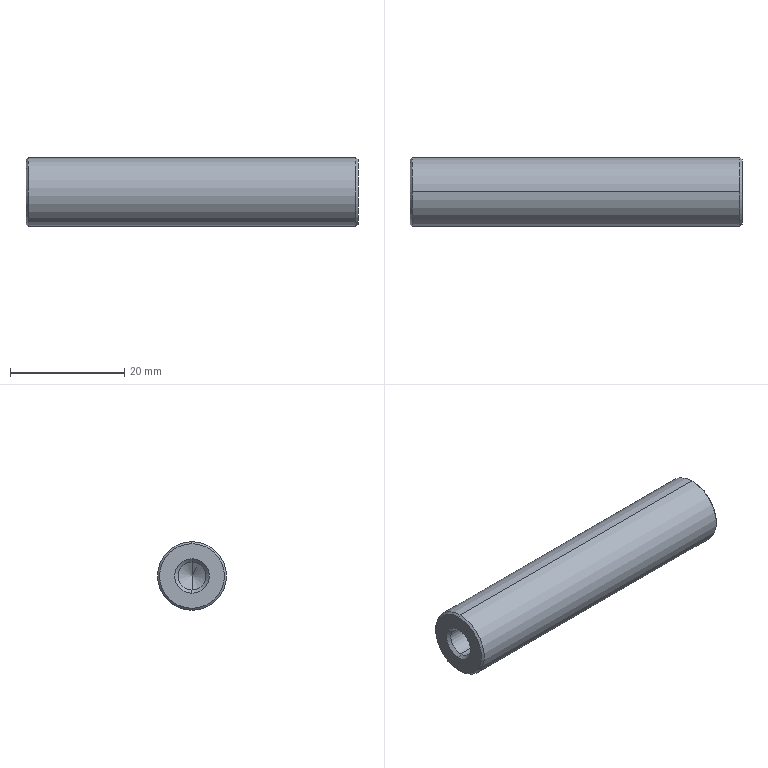Part | NX | features BREP 1 | 1 solid | 14 faces | box 58 x 12 x 12 mm | volume 6309 mm3 | cone 8 | cylinder 4 | plane 2 | commonest cylinder face diameters 4.917 x2 12 x2
STEP:
#1=CARTESIAN_POINT('',(58.,0.,5.646));
#2=VERTEX_POINT('',#1);
#3=CARTESIAN_POINT('',(58.,0.,-5.646));
#4=VERTEX_POINT('',#3);
#5=CARTESIAN_POINT('',(58.,0.,0.));
#6=DIRECTION('',(-1.,0.,0.));
#7=DIRECTION('',(0.,0.,1.));
#8=AXIS2_PLACEMENT_3D('',#5,#6,#7);
#9=CIRCLE('',#8,5.646);
#10=EDGE_CURVE('',#2,#4,#9,.T.);
#11=ORIENTED_EDGE('',*,*,#10,.T.);
#12=CARTESIAN_POINT('',(57.646,0.,-6.));
#13=VERTEX_POINT('',#12);
#14=CARTESIAN_POINT('',(58.,0.,-5.646));
#15=DIRECTION('',(-0.7071,0.,-0.7071));
#16=VECTOR('',#15,1000.);
#17=LINE('',#14,#16);
#18=EDGE_CURVE('',#4,#13,#17,.T.);
#19=ORIENTED_EDGE('',*,*,#18,.T.);
#20=CARTESIAN_POINT('',(57.646,0.,6.));
#21=VERTEX_POINT('',#20);
#22=CARTESIAN_POINT('',(57.646,0.,0.));
#23=DIRECTION('',(-1.,0.,0.));
#24=DIRECTION('',(0.,0.,1.));
#25=AXIS2_PLACEMENT_3D('',#22,#23,#24);
#26=CIRCLE('',#25,6.);
#27=EDGE_CURVE('',#21,#13,#26,.T.);
#28=ORIENTED_EDGE('',*,*,#27,.F.);
#29=CARTESIAN_POINT('',(58.,0.,5.646));
#30=DIRECTION('',(-0.7071,0.,0.7071));
#31=VECTOR('',#30,1000.);
#32=LINE('',#29,#31);
#33=EDGE_CURVE('',#2,#21,#32,.T.);
#34=ORIENTED_EDGE('',*,*,#33,.F.);
#35=EDGE_LOOP('',(#11,#19,#28,#34));
#36=FACE_BOUND('',#35,.T.);
#37=CARTESIAN_POINT('',(58.,0.,0.));
#38=DIRECTION('',(-1.,0.,0.));
#39=DIRECTION('',(0.,0.,-1.));
#40=AXIS2_PLACEMENT_3D('',#37,#38,#39);
#41=CONICAL_SURFACE('',#40,5.646,0.7854);
#42=ADVANCED_FACE('',(#36),#41,.T.);
#43=ORIENTED_EDGE('',*,*,#27,.T.);
#44=CARTESIAN_POINT('',(0.3536,0.,-6.));
#45=VERTEX_POINT('',#44);
#46=CARTESIAN_POINT('',(58.,0.,-6.));
#47=DIRECTION('',(-1.,0.,0.));
#48=VECTOR('',#47,1000.);
#49=LINE('',#46,#48);
#50=EDGE_CURVE('',#13,#45,#49,.T.);
#51=ORIENTED_EDGE('',*,*,#50,.T.);
#52=CARTESIAN_POINT('',(0.3536,0.,6.));
#53=VERTEX_POINT('',#52);
#54=CARTESIAN_POINT('',(0.3536,0.,0.));
#55=DIRECTION('',(-1.,0.,0.));
#56=DIRECTION('',(0.,0.,1.));
#57=AXIS2_PLACEMENT_3D('',#54,#55,#56);
#58=CIRCLE('',#57,6.);
#59=EDGE_CURVE('',#53,#45,#58,.T.);
#60=ORIENTED_EDGE('',*,*,#59,.F.);
#61=CARTESIAN_POINT('',(58.,0.,6.));
#62=DIRECTION('',(-1.,0.,0.));
#63=VECTOR('',#62,1000.);
#64=LINE('',#61,#63);
#65=EDGE_CURVE('',#21,#53,#64,.T.);
#66=ORIENTED_EDGE('',*,*,#65,.F.);
#67=EDGE_LOOP('',(#43,#51,#60,#66));
#68=FACE_BOUND('',#67,.T.);
#69=CARTESIAN_POINT('',(58.,0.,0.));
#70=DIRECTION('',(-1.,0.,0.));
#71=DIRECTION('',(0.,0.,-1.));
#72=AXIS2_PLACEMENT_3D('',#69,#70,#71);
#73=CYLINDRICAL_SURFACE('',#72,6.);
#74=ADVANCED_FACE('',(#68),#73,.T.);
#75=CARTESIAN_POINT('',(0.,0.,5.646));
#76=VERTEX_POINT('',#75);
#77=CARTESIAN_POINT('',(0.,0.,-5.646));
#78=VERTEX_POINT('',#77);
#79=CARTESIAN_POINT('',(0.,0.,0.));
#80=DIRECTION('',(-1.,0.,0.));
#81=DIRECTION('',(0.,0.,1.));
#82=AXIS2_PLACEMENT_3D('',#79,#80,#81);
#83=CIRCLE('',#82,5.646);
#84=EDGE_CURVE('',#76,#78,#83,.T.);
#85=ORIENTED_EDGE('',*,*,#84,.F.);
#86=CARTESIAN_POINT('',(0.3536,0.,6.));
#87=DIRECTION('',(0.7071,0.,0.7071));
#88=VECTOR('',#87,1000.);
#89=LINE('',#86,#88);
#90=EDGE_CURVE('',#53,#76,#89,.F.);
#91=ORIENTED_EDGE('',*,*,#90,.F.);
#92=ORIENTED_EDGE('',*,*,#59,.T.);
#93=CARTESIAN_POINT('',(0.3536,0.,-6.));
#94=DIRECTION('',(0.7071,0.,-0.7071));
#95=VECTOR('',#94,1000.);
#96=LINE('',#93,#95);
#97=EDGE_CURVE('',#45,#78,#96,.F.);
#98=ORIENTED_EDGE('',*,*,#97,.T.);
#99=EDGE_LOOP('',(#85,#91,#92,#98));
#100=FACE_BOUND('',#99,.T.);
#101=CARTESIAN_POINT('',(0.3536,0.,0.));
#102=DIRECTION('',(1.,0.,0.));
#103=DIRECTION('',(0.,0.,1.));
#104=AXIS2_PLACEMENT_3D('',#101,#102,#103);
#105=CONICAL_SURFACE('',#104,6.,0.7854);
#106=ADVANCED_FACE('',(#100),#105,.T.);
#107=CARTESIAN_POINT('',(0.5415,0.,-2.458));
#108=VERTEX_POINT('',#107);
#109=CARTESIAN_POINT('',(0.5415,0.,2.458));
#110=VERTEX_POINT('',#109);
#111=CARTESIAN_POINT('',(0.5415,0.,0.));
#112=DIRECTION('',(-1.,0.,0.));
#113=DIRECTION('',(0.,0.,1.));
#114=AXIS2_PLACEMENT_3D('',#111,#112,#113);
#115=CIRCLE('',#114,2.458);
#116=EDGE_CURVE('',#108,#110,#115,.T.);
#117=ORIENTED_EDGE('',*,*,#116,.F.);
#118=CARTESIAN_POINT('',(0.,0.,-3.));
#119=VERTEX_POINT('',#118);
#120=CARTESIAN_POINT('',(0.,0.,-3.));
#121=DIRECTION('',(-0.7071,0.,-0.7071));
#122=VECTOR('',#121,1000.);
#123=LINE('',#120,#122);
#124=EDGE_CURVE('',#108,#119,#123,.T.);
#125=ORIENTED_EDGE('',*,*,#124,.T.);
#126=CARTESIAN_POINT('',(0.,0.,3.));
#127=VERTEX_POINT('',#126);
#128=CARTESIAN_POINT('',(0.,0.,0.));
#129=DIRECTION('',(-1.,0.,0.));
#130=DIRECTION('',(0.,0.,1.));
#131=AXIS2_PLACEMENT_3D('',#128,#129,#130);
#132=CIRCLE('',#131,3.);
#133=EDGE_CURVE('',#119,#127,#132,.T.);
#134=ORIENTED_EDGE('',*,*,#133,.T.);
#135=CARTESIAN_POINT('',(0.,0.,3.));
#136=DIRECTION('',(-0.7071,0.,0.7071));
#137=VECTOR('',#136,1000.);
#138=LINE('',#135,#137);
#139=EDGE_CURVE('',#110,#127,#138,.T.);
#140=ORIENTED_EDGE('',*,*,#139,.F.);
#141=EDGE_LOOP('',(#117,#125,#134,#140));
#142=FACE_BOUND('',#141,.T.);
#143=CARTESIAN_POINT('',(0.,0.,0.));
#144=DIRECTION('',(-1.,0.,0.));
#145=DIRECTION('',(0.,0.,-1.));
#146=AXIS2_PLACEMENT_3D('',#143,#144,#145);
#147=CONICAL_SURFACE('',#146,3.,0.7854);
#148=ADVANCED_FACE('',(#142),#147,.F.);
#149=CARTESIAN_POINT('',(12.325,0.,-2.458));
#150=VERTEX_POINT('',#149);
#151=CARTESIAN_POINT('',(12.325,0.,2.458));
#152=VERTEX_POINT('',#151);
#153=CARTESIAN_POINT('',(12.325,0.,0.));
#154=DIRECTION('',(-1.,0.,0.));
#155=DIRECTION('',(0.,0.,1.));
#156=AXIS2_PLACEMENT_3D('',#153,#154,#155);
#157=CIRCLE('',#156,2.458);
#158=EDGE_CURVE('',#150,#152,#157,.T.);
#159=ORIENTED_EDGE('',*,*,#158,.F.);
#160=CARTESIAN_POINT('',(58.,0.,-2.458));
#161=DIRECTION('',(-1.,0.,0.));
#162=VECTOR('',#161,1000.);
#163=LINE('',#160,#162);
#164=EDGE_CURVE('',#150,#108,#163,.T.);
#165=ORIENTED_EDGE('',*,*,#164,.T.);
#166=ORIENTED_EDGE('',*,*,#116,.T.);
#167=CARTESIAN_POINT('',(58.,0.,2.458));
#168=DIRECTION('',(-1.,0.,0.));
#169=VECTOR('',#168,1000.);
#170=LINE('',#167,#169);
#171=EDGE_CURVE('',#152,#110,#170,.T.);
#172=ORIENTED_EDGE('',*,*,#171,.F.);
#173=EDGE_LOOP('',(#159,#165,#166,#172));
#174=FACE_BOUND('',#173,.T.);
#175=CARTESIAN_POINT('',(58.,0.,0.));
#176=DIRECTION('',(-1.,0.,0.));
#177=DIRECTION('',(0.,0.,-1.));
#178=AXIS2_PLACEMENT_3D('',#175,#176,#177);
#179=CYLINDRICAL_SURFACE('',#178,2.458);
#180=ADVANCED_FACE('',(#174),#179,.F.);
#181=CARTESIAN_POINT('',(13.803,0.,0.));
#182=VERTEX_POINT('',#181);
#183=CARTESIAN_POINT('',(12.325,0.,2.458));
#184=DIRECTION('',(-0.515,0.,0.8572));
#185=VECTOR('',#184,1000.);
#186=LINE('',#183,#185);
#187=EDGE_CURVE('',#182,#152,#186,.T.);
#188=ORIENTED_EDGE('',*,*,#187,.F.);
#189=CARTESIAN_POINT('',(12.325,0.,-2.458));
#190=DIRECTION('',(-0.515,0.,-0.8572));
#191=VECTOR('',#190,1000.);
#192=LINE('',#189,#191);
#193=EDGE_CURVE('',#182,#150,#192,.T.);
#194=ORIENTED_EDGE('',*,*,#193,.T.);
#195=ORIENTED_EDGE('',*,*,#158,.T.);
#196=EDGE_LOOP('',(#188,#194,#195));
#197=FACE_BOUND('',#196,.T.);
#198=CARTESIAN_POINT('',(12.325,0.,0.));
#199=DIRECTION('',(-1.,0.,0.));
#200=DIRECTION('',(0.,0.,-1.));
#201=AXIS2_PLACEMENT_3D('',#198,#199,#200);
#202=CONICAL_SURFACE('',#201,2.458,1.03);
#203=ADVANCED_FACE('',(#197),#202,.F.);
#204=ORIENTED_EDGE('',*,*,#193,.F.);
#205=ORIENTED_EDGE('',*,*,#187,.T.);
#206=CARTESIAN_POINT('',(12.325,0.,0.));
#207=DIRECTION('',(-1.,0.,0.));
#208=DIRECTION('',(0.,0.,1.));
#209=AXIS2_PLACEMENT_3D('',#206,#207,#208);
#210=CIRCLE('',#209,2.458);
#211=EDGE_CURVE('',#152,#150,#210,.T.);
#212=ORIENTED_EDGE('',*,*,#211,.T.);
#213=EDGE_LOOP('',(#204,#205,#212));
#214=FACE_BOUND('',#213,.T.);
#215=CARTESIAN_POINT('',(12.325,0.,0.));
#216=DIRECTION('',(-1.,0.,0.));
#217=DIRECTION('',(0.,0.,-1.));
#218=AXIS2_PLACEMENT_3D('',#215,#216,#217);
#219=CONICAL_SURFACE('',#218,2.458,1.03);
#220=ADVANCED_FACE('',(#214),#219,.F.);
#221=ORIENTED_EDGE('',*,*,#164,.F.);
#222=ORIENTED_EDGE('',*,*,#211,.F.);
#223=ORIENTED_EDGE('',*,*,#171,.T.);
#224=CARTESIAN_POINT('',(0.5415,0.,0.));
#225=DIRECTION('',(-1.,0.,0.));
#226=DIRECTION('',(0.,0.,1.));
#227=AXIS2_PLACEMENT_3D('',#224,#225,#226);
#228=CIRCLE('',#227,2.458);
#229=EDGE_CURVE('',#110,#108,#228,.T.);
#230=ORIENTED_EDGE('',*,*,#229,.T.);
#231=EDGE_LOOP('',(#221,#222,#223,#230));
#232=FACE_BOUND('',#231,.T.);
#233=CARTESIAN_POINT('',(58.,0.,0.));
#234=DIRECTION('',(-1.,0.,0.));
#235=DIRECTION('',(0.,0.,-1.));
#236=AXIS2_PLACEMENT_3D('',#233,#234,#235);
#237=CYLINDRICAL_SURFACE('',#236,2.458);
#238=ADVANCED_FACE('',(#232),#237,.F.);
#239=ORIENTED_EDGE('',*,*,#124,.F.);
#240=ORIENTED_EDGE('',*,*,#229,.F.);
#241=ORIENTED_EDGE('',*,*,#139,.T.);
#242=CARTESIAN_POINT('',(0.,0.,0.));
#243=DIRECTION('',(-1.,0.,0.));
#244=DIRECTION('',(0.,0.,1.));
#245=AXIS2_PLACEMENT_3D('',#242,#243,#244);
#246=CIRCLE('',#245,3.);
#247=EDGE_CURVE('',#127,#119,#246,.T.);
#248=ORIENTED_EDGE('',*,*,#247,.T.);
#249=EDGE_LOOP('',(#239,#240,#241,#248));
#250=FACE_BOUND('',#249,.T.);
#251=CARTESIAN_POINT('',(0.,0.,0.));
#252=DIRECTION('',(-1.,0.,0.));
#253=DIRECTION('',(0.,0.,-1.));
#254=AXIS2_PLACEMENT_3D('',#251,#252,#253);
#255=CONICAL_SURFACE('',#254,3.,0.7854);
#256=ADVANCED_FACE('',(#250),#255,.F.);
#257=ORIENTED_EDGE('',*,*,#247,.F.);
#258=ORIENTED_EDGE('',*,*,#133,.F.);
#259=EDGE_LOOP('',(#257,#258));
#260=FACE_BOUND('',#259,.T.);
#261=CARTESIAN_POINT('',(0.,0.,0.));
#262=DIRECTION('',(-1.,0.,0.));
#263=DIRECTION('',(0.,0.,1.));
#264=AXIS2_PLACEMENT_3D('',#261,#262,#263);
#265=CIRCLE('',#264,5.646);
#266=EDGE_CURVE('',#78,#76,#265,.T.);
#267=ORIENTED_EDGE('',*,*,#266,.T.);
#268=ORIENTED_EDGE('',*,*,#84,.T.);
#269=EDGE_LOOP('',(#267,#268));
#270=FACE_BOUND('',#269,.T.);
#271=CARTESIAN_POINT('',(0.,3.,0.));
#272=DIRECTION('',(1.,0.,0.));
#273=DIRECTION('',(0.,0.,1.));
#274=AXIS2_PLACEMENT_3D('',#271,#272,#273);
#275=PLANE('',#274);
#276=ADVANCED_FACE('',(#260,#270),#275,.F.);
#277=ORIENTED_EDGE('',*,*,#90,.T.);
#278=ORIENTED_EDGE('',*,*,#266,.F.);
#279=ORIENTED_EDGE('',*,*,#97,.F.);
#280=CARTESIAN_POINT('',(0.3536,0.,0.));
#281=DIRECTION('',(-1.,0.,0.));
#282=DIRECTION('',(0.,0.,1.));
#283=AXIS2_PLACEMENT_3D('',#280,#281,#282);
#284=CIRCLE('',#283,6.);
#285=EDGE_CURVE('',#45,#53,#284,.T.);
#286=ORIENTED_EDGE('',*,*,#285,.T.);
#287=EDGE_LOOP('',(#277,#278,#279,#286));
#288=FACE_BOUND('',#287,.T.);
#289=CARTESIAN_POINT('',(0.3536,0.,0.));
#290=DIRECTION('',(1.,0.,0.));
#291=DIRECTION('',(0.,0.,1.));
#292=AXIS2_PLACEMENT_3D('',#289,#290,#291);
#293=CONICAL_SURFACE('',#292,6.,0.7854);
#294=ADVANCED_FACE('',(#288),#293,.T.);
#295=ORIENTED_EDGE('',*,*,#50,.F.);
#296=CARTESIAN_POINT('',(57.646,0.,0.));
#297=DIRECTION('',(-1.,0.,0.));
#298=DIRECTION('',(0.,0.,1.));
#299=AXIS2_PLACEMENT_3D('',#296,#297,#298);
#300=CIRCLE('',#299,6.);
#301=EDGE_CURVE('',#13,#21,#300,.T.);
#302=ORIENTED_EDGE('',*,*,#301,.T.);
#303=ORIENTED_EDGE('',*,*,#65,.T.);
#304=ORIENTED_EDGE('',*,*,#285,.F.);
#305=EDGE_LOOP('',(#295,#302,#303,#304));
#306=FACE_BOUND('',#305,.T.);
#307=CARTESIAN_POINT('',(58.,0.,0.));
#308=DIRECTION('',(-1.,0.,0.));
#309=DIRECTION('',(0.,0.,-1.));
#310=AXIS2_PLACEMENT_3D('',#307,#308,#309);
#311=CYLINDRICAL_SURFACE('',#310,6.);
#312=ADVANCED_FACE('',(#306),#311,.T.);
#313=ORIENTED_EDGE('',*,*,#18,.F.);
#314=CARTESIAN_POINT('',(58.,0.,0.));
#315=DIRECTION('',(-1.,0.,0.));
#316=DIRECTION('',(0.,0.,1.));
#317=AXIS2_PLACEMENT_3D('',#314,#315,#316);
#318=CIRCLE('',#317,5.646);
#319=EDGE_CURVE('',#4,#2,#318,.T.);
#320=ORIENTED_EDGE('',*,*,#319,.T.);
#321=ORIENTED_EDGE('',*,*,#33,.T.);
#322=ORIENTED_EDGE('',*,*,#301,.F.);
#323=EDGE_LOOP('',(#313,#320,#321,#322));
#324=FACE_BOUND('',#323,.T.);
#325=CARTESIAN_POINT('',(58.,0.,0.));
#326=DIRECTION('',(-1.,0.,0.));
#327=DIRECTION('',(0.,0.,-1.));
#328=AXIS2_PLACEMENT_3D('',#325,#326,#327);
#329=CONICAL_SURFACE('',#328,5.646,0.7854);
#330=ADVANCED_FACE('',(#324),#329,.T.);
#331=ORIENTED_EDGE('',*,*,#10,.F.);
#332=ORIENTED_EDGE('',*,*,#319,.F.);
#333=EDGE_LOOP('',(#331,#332));
#334=FACE_BOUND('',#333,.T.);
#335=CARTESIAN_POINT('',(58.,5.646,0.));
#336=DIRECTION('',(-1.,0.,0.));
#337=DIRECTION('',(0.,0.,-1.));
#338=AXIS2_PLACEMENT_3D('',#335,#336,#337);
#339=PLANE('',#338);
#340=ADVANCED_FACE('',(#334),#339,.F.);
#341=CLOSED_SHELL('',(#42,#74,#106,#148,#180,#203,#220,#238,#256,#276,#294,#312,#330,#340));
#342=MANIFOLD_SOLID_BREP('',#341);
#343=(LENGTH_UNIT()NAMED_UNIT(*)SI_UNIT(.MILLI.,.METRE.));
#344=UNCERTAINTY_MEASURE_WITH_UNIT(LENGTH_MEASURE(0.00001),#343,'','');
#345=(NAMED_UNIT(*)PLANE_ANGLE_UNIT()SI_UNIT($,.RADIAN.));
#346=(NAMED_UNIT(*)SI_UNIT($,.STERADIAN.)SOLID_ANGLE_UNIT());
#347=(GEOMETRIC_REPRESENTATION_CONTEXT(3)GLOBAL_UNCERTAINTY_ASSIGNED_CONTEXT((#344))GLOBAL_UNIT_ASSIGNED_CONTEXT((#343,#345,#346))REPRESENTATION_CONTEXT('',''));
#348=ADVANCED_BREP_SHAPE_REPRESENTATION('',(#342),#347);